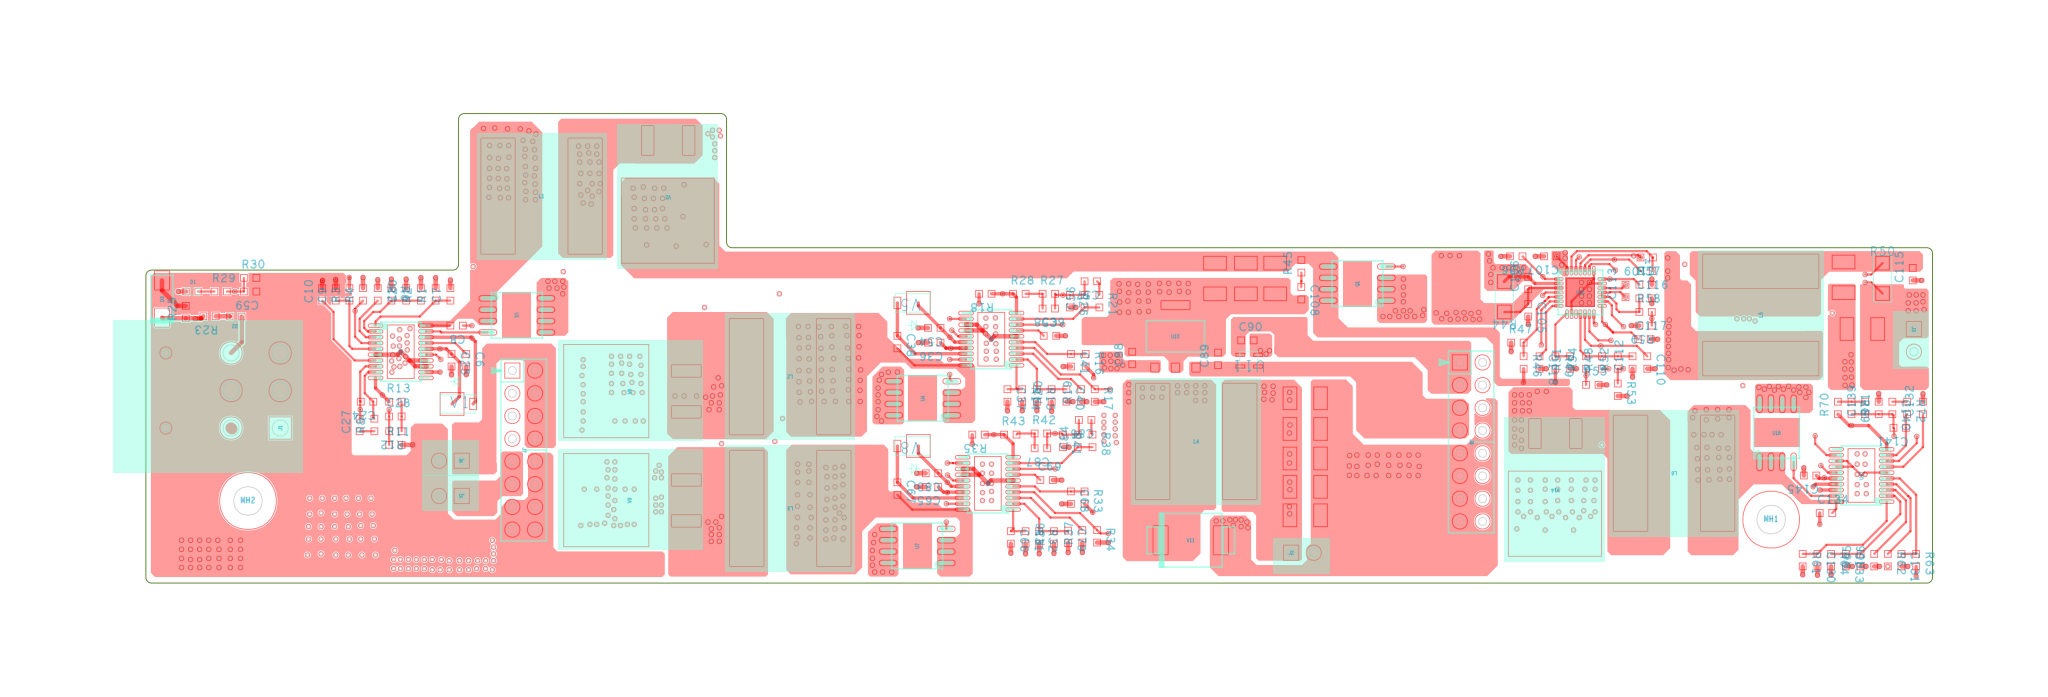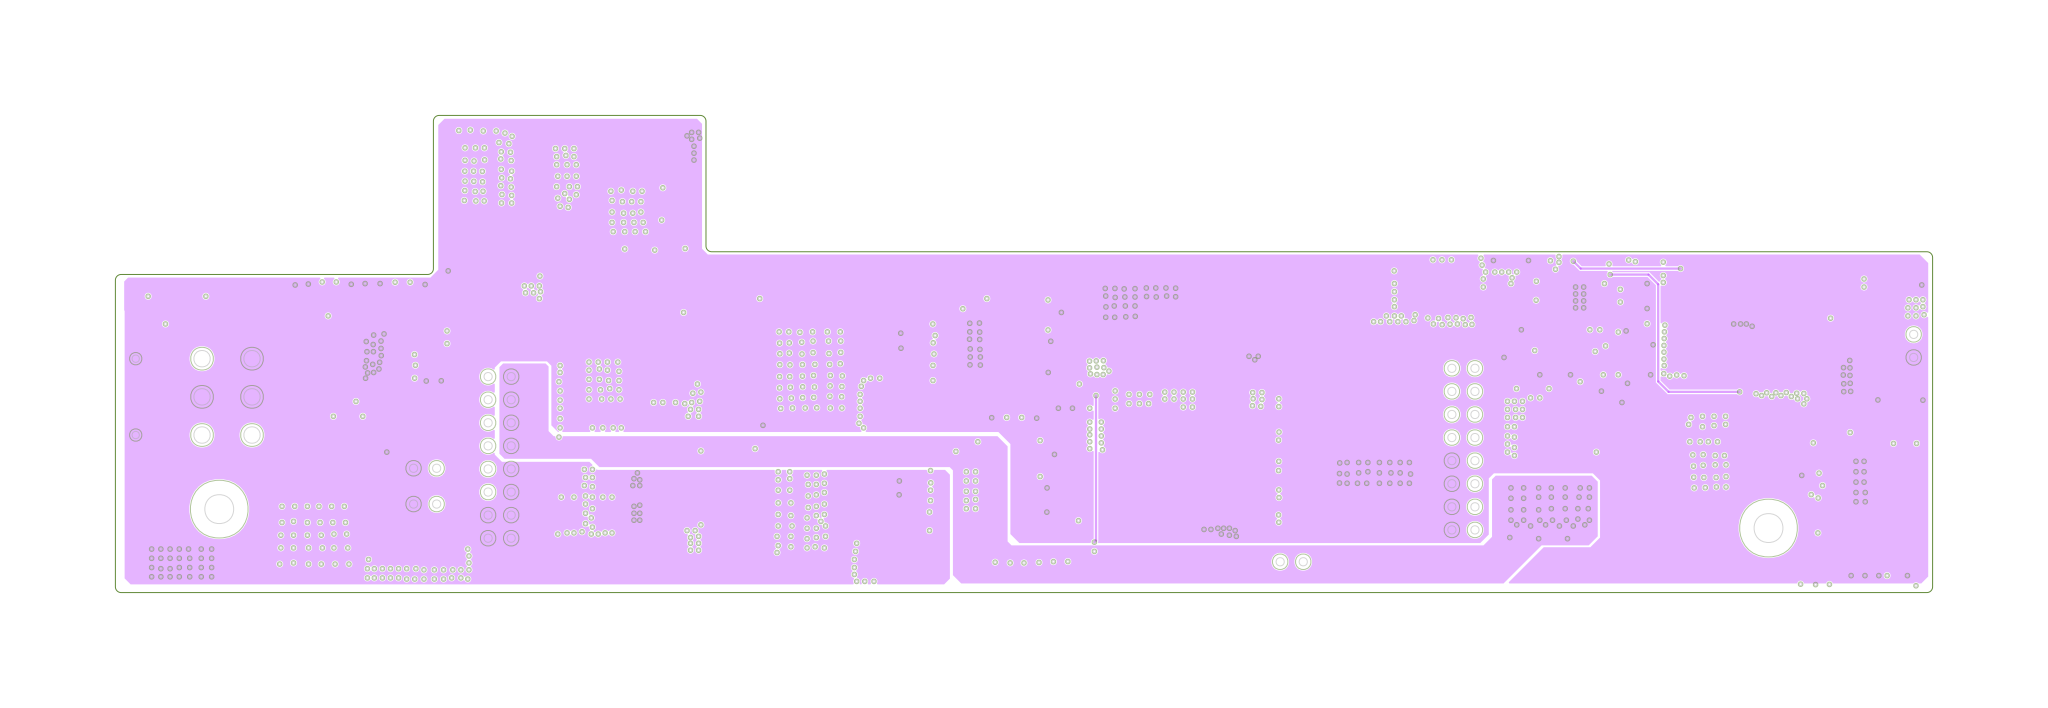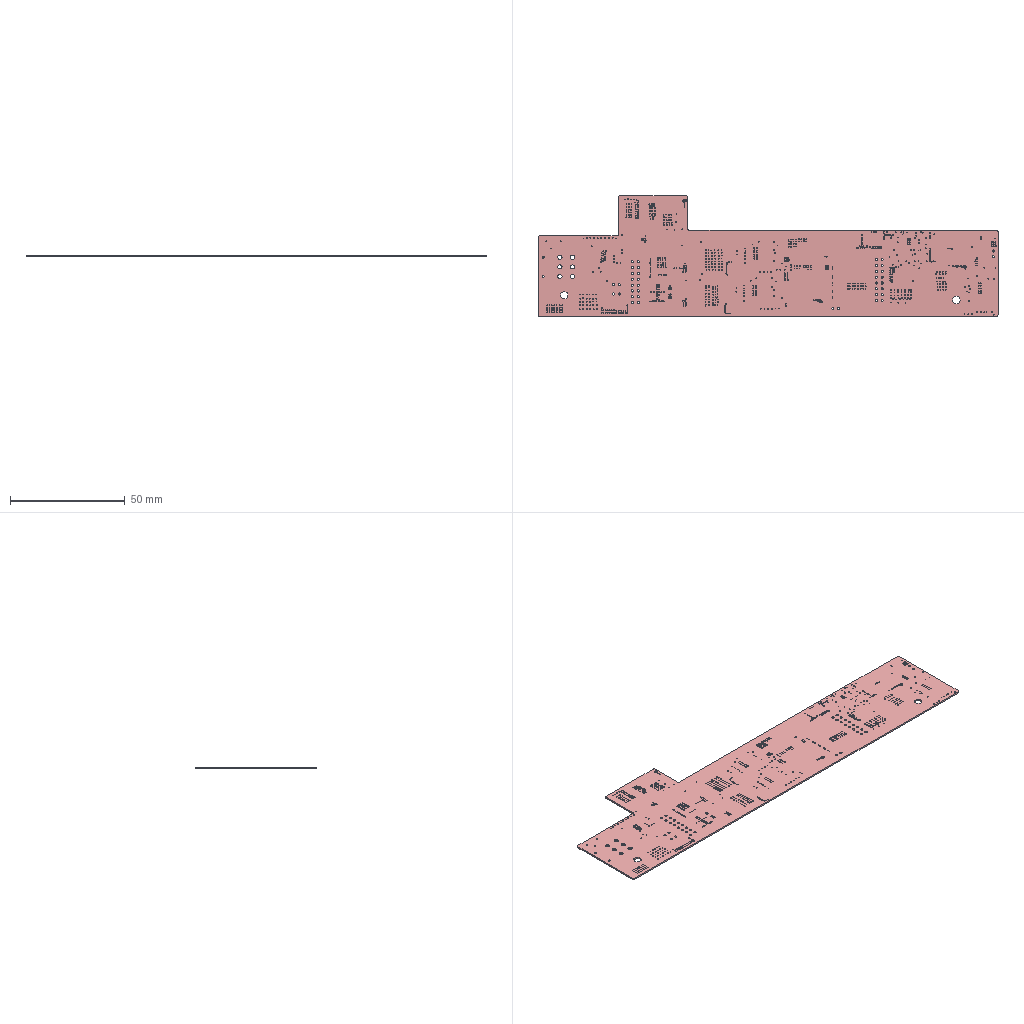Circuit board layout | Cadence Allegro | box 200 x 52.5 x 0.7 mm
Layer stack:
# Cadence Allegro layer stack of  (unit mm; from the constraint file cross-section; dielectric type: 0 not recorded (Allegro does not mark core vs prepreg), 3 surface material)
index,name,kind,layer,copper_thickness_mm,dielectric_type,dielectric_thickness_mm,dielectric_material,dielectric_constant
0,Top Surface,other,,,,,,
1,TOP,copper,TOP,0.0305,,,,
2,Dielectric1,dielectric,,,0,0.2032,FR-4,4.5
3,L2,copper,L2,0.0305,,,,
4,Dielectric2,dielectric,,,0,0.2032,FR-4,4.5
5,L3,copper,L3,0.0305,,,,
6,Dielectric3,dielectric,,,0,0.2032,FR-4,4.5
7,BOTTOM,copper,BOTTOM,0.0305,,,,
8,Bottom Surface,other,,,,,,
# drill layer pairs: low layer,high layer
drill_pair,TOP,BOTTOM
Part placement:
REFDES,COMP_VALUE,SYM_NAME,SYM_X,SYM_Y,SYM_ROTATE,SYM_MIRROR
C1,22uF,C1210,-2818.000,-2737.000,270.000,YES
C6,1uF,C0603,-2585.000,-1952.500,270.000,NO
C7,0.1uF,R0603,-2655.000,-1662.500,90.000,NO
C8,0.1uF,C0603,-2627.500,-1800.000,180.000,NO
C9,330pF,C0603,-3160.000,-1662.500,90.000,NO
C10,0.1uF,C0603,-3220.000,-1662.500,90.000,NO
C11,47uF,C1210,722.000,-1588.000,270.000,NO
C12,47uF,C1210,987.000,-1588.000,270.000,NO
C13,47uF,C1210,-1527.000,-1508.000,90.000,YES
C14,47uF,C1210,858.000,-1588.000,270.000,NO
C15,47uF,C1210,-1561.992,-1041.535,180.000,YES
C16,47uF,C1210,-1561.992,-1179.535,180.000,YES
C17,47uF,C1210,-1561.992,-1317.535,180.000,YES
C18,47uF,C1210,-1797.000,-1508.000,90.000,YES
C19,47uF,C1210,-1662.000,-1508.000,90.000,YES
C20,0.1uF,C0603,-2850.000,-1662.500,90.000,NO
C24,2200pF,C0603,-3022.500,-2135.000,180.000,NO
C25,1uF,C0603,-2650.000,-1952.500,270.000,NO
C26,NO-POP,C0603,-2422.500,-1540.000,0.000,YES
C27,4700pF,C0603,-3055.000,-2237.500,90.000,NO
C28,NO-POP,C0603,-2897.500,-2200.000,0.000,NO
C31,22uF,C1210,-2548.000,-2737.000,270.000,YES
C36,1uF,C0603,-522.500,-1875.000,180.000,NO
C37,0.1uF,R0603,-200.000,-2107.500,270.000,NO
C38,0.1uF,C0603,-685.000,-1872.500,270.000,NO
C39,0.1uF,C0603,-12.500,-1845.000,0.000,NO
C40,0.1uF,R0603,60.000,-2107.500,270.000,NO
C41,330pF,C0603,80.000,-1952.500,270.000,NO
C42,47uF,C1210,-1863.000,-1793.000,270.000,YES
C43,47uF,C1210,-2133.000,-1792.000,270.000,YES
C44,47uF,C1210,-2083.000,-1973.000,0.000,YES
C45,47uF,C1210,-2268.000,-1792.000,270.000,YES
C46,47uF,C1210,-1782.000,-2233.000,90.000,YES
C47,47uF,C1210,-1912.000,-2233.000,90.000,YES
C48,47uF,C1210,-1998.000,-1792.000,270.000,YES
C49,47uF,C1210,-2083.000,-2233.000,0.000,YES
C50,47uF,C1210,-2083.000,-2103.000,0.000,YES
C54,1uF,C0603,-522.500,-1810.000,180.000,NO
C55,0.1uF,C0603,-1177.500,-1700.000,180.000,YES
C56,2200pF,C0603,140.000,-1692.500,90.000,NO
C57,4700pF,C0603,167.500,-1605.000,180.000,NO
C58,0.01uF,C0603,-17.500,-1725.000,180.000,NO
C59,0.1uF,C0603,-3537.500,-1650.000,180.000,NO
C60,22uF,C1210,-2683.000,-2737.000,270.000,YES
C65,1uF,C0603,-532.500,-2510.000,180.000,NO
C66,0.1uF,R0603,-185.000,-2732.500,270.000,NO
C67,0.1uF,C0603,-685.000,-2517.500,270.000,NO
C68,330pF,C0603,80.000,-2557.500,270.000,NO
C69,0.1uF,C0603,-27.500,-2480.000,0.000,NO
C70,47uF,C1210,-1742.000,-2798.000,90.000,YES
C71,47uF,C1210,-1877.000,-2798.000,90.000,YES
C72,47uF,C1210,-2007.000,-2798.000,90.000,YES
C73,47uF,C1210,-2137.000,-2798.000,90.000,YES
C74,47uF,C1210,-2083.000,-2588.000,0.000,YES
C75,47uF,C1210,-1812.000,-2597.000,180.000,YES
C76,47uF,C1210,-1812.000,-2447.000,180.000,YES
C77,47uF,C1210,-1607.000,-2798.000,90.000,YES
C78,47uF,C1210,-2083.000,-2438.000,0.000,YES
C79,0.1uF,R0603,67.500,-2730.000,270.000,NO
C83,1uF,C0603,-532.500,-2450.000,180.000,NO
C84,2200pF,C0603,110.000,-2307.500,90.000,NO
C85,0.1uF,C0603,-1197.500,-2340.000,180.000,YES
C86,4700pF,C0603,142.500,-2215.000,180.000,NO
C87,0.01uF,C0603,-52.500,-2340.000,180.000,NO
C88,0.1uF,C0603,350.000,-1942.500,90.000,NO
C89,0.1uF,C0603,728.000,-1946.500,90.000,NO
C90,0.1uF,C0603,857.500,-1865.000,0.000,NO
C91,47uF/25V,C1210,376.000,-2449.000,90.000,YES
C92,47uF/25V,C1210,239.000,-2448.000,90.000,YES
C93,100uF/10V,C1210,1108.000,-2248.000,0.000,NO
C94,100uF/10V,C1210,1108.000,-2113.000,0.000,NO
C95,100uF/10V,C1210,1108.000,-2628.000,0.000,NO
C96,100uF/10V,C1210,1107.000,-2638.000,180.000,YES
C97,100uF/10V,C1210,1107.000,-2133.000,180.000,YES
C98,100uF/10V,C1210,1107.000,-2383.000,180.000,YES
C99,100uF/10V,C1210,1107.000,-2508.000,180.000,YES
C100,100uF/10V,C1210,1108.000,-2503.000,0.000,NO
C101,100uF/10V,C1210,1108.000,-2378.000,0.000,NO
C102,100uF/10V,C1210,1107.000,-2258.000,180.000,YES
C103,10uF,C1210,3338.000,-1832.000,180.000,YES
C104,10uF,C1210,3338.000,-1962.000,180.000,YES
C105,0.1uF,R0603,2095.000,-1732.500,270.000,NO
C106,0.1uF,R0603,2095.000,-1612.500,90.000,NO
C107,0.1uF,C0603,2192.500,-1495.000,180.000,NO
C108,2.2uF,C0603,1095.000,-1657.500,270.000,NO
C109,0.1uF,C0603,2617.500,-1500.000,180.000,NO
C110,1uF,C0603,2620.000,-1962.500,270.000,NO
C111,10uF,C1210,3492.000,-1583.000,270.000,NO
C112,1uF,C0603,2555.000,-1962.500,90.000,NO
C113,0.1uF,C0603,2524.000,-1647.500,90.000,NO
C114,10uF,C1210,3572.000,-1822.000,180.000,NO
C115,0.1uF,C0603,3790.000,-1573.500,90.000,NO
C116,0.1uF,C0603,2612.500,-1680.000,0.000,NO
C117,100pF,C0603,2607.500,-1860.000,0.000,NO
C118,0.47uF,C0603,2145.000,-1962.500,270.000,NO
C119,47uF,C1210,1611.000,-2626.000,270.000,YES
C120,47uF,C1210,2682.000,-2762.000,90.000,YES
C121,47uF,C1210,1345.000,-2627.000,270.000,YES
C122,47uF,C1210,1478.000,-2626.000,270.000,YES
C123,47uF,C1210,2037.000,-2762.000,90.000,YES
C124,47uF,C1210,2167.000,-2762.000,90.000,YES
C125,47uF,C1210,2297.000,-2762.000,90.000,YES
C126,47uF,C1210,2427.000,-2762.000,90.000,YES
C129,22uF,C1210,3338.000,-2087.000,180.000,YES
C130,0.1uF,R0603,3370.000,-2832.500,270.000,NO
C131,330pF,C0603,3740.000,-2832.500,270.000,NO
C132,0.1uF,C0603,3835.000,-2162.500,90.000,NO
C133,0.1uF,R0603,3495.000,-2832.500,270.000,NO
C134,0.1uF,C0603,3407.500,-2625.000,0.000,NO
C135,0.1uF,C0603,3360.000,-2342.500,90.000,YES
C139,0.01uF,C0603,3580.000,-2162.500,90.000,NO
C140,4700pF,C0603,3700.000,-2162.500,270.000,NO
C141,2200pF,C0603,3732.500,-2250.000,180.000,NO
C142,1uF,C0603,2805.000,-2837.500,90.000,YES
C145,1uF,C0603,3337.500,-2460.000,180.000,NO
C146,47uF,C1210,2557.000,-2762.000,90.000,YES
D1,bat54-02v-gs08,SOD_523,-3793.500,-1650.000,0.000,NO
D2,bat54-02v-gs08,SOD_523,-3600.500,-1760.000,180.000,NO
D3,Zener_ZMM5.1,SOD_123,-3926.000,-1683.110,90.000,NO
D4,bat54-02v-gs08,SOD_523,2616.500,-1560.000,0.000,NO
D5,SMCJ14A-13-F,DO-214AB,-3810.000,-2542.000,90.000,YES
F1,F_6.0A,FUSEFOLDER-OMNI-BLOK,-3182.000,-1987.000,90.000,YES
J1,PoweIn,HDR4MM2_2X3,-3405.000,-2251.000,90.000,NO
J2,+5V,HDR2MM54_1X2,1050.000,-2800.000,0.000,NO
J3,Battery---12V,HDR2MM54_1X2,3795.000,-1815.000,270.000,NO
J5,+5V,HDR2MM54_1X2,-2605.000,-2550.000,180.000,NO
J6,+12V,HDR2MM54_1X2,-2605.000,-2395.000,180.000,NO
J7,HEADER 8X2,HDR2MM54_2X8,-2382.000,-1998.000,270.000,NO
J8,HEADER 8X2,HDR2MM54_2X8,1794.000,-1962.000,270.000,NO
L1,10uH,L-12X12X7,-2253.071,-1230.000,0.000,NO
L2,10uH,L-12X12X7,-1158.071,-2025.000,180.000,NO
L3,10uH,L-12X12X7,-1156.929,-2605.000,180.000,NO
L4,100uH,L-12X14X8,631.929,-2310.000,0.000,NO
L5,10uH,L-12X12X7,3120.000,-1753.071,90.000,NO
L6,10uH,L-12X12X7,2738.071,-2450.000,180.000,NO
MH1,MH_3MM,MHP125-250,3166.000,-2654.000,0.000,NO
MH2,MH_3MM,MHP125-250,-3547.000,-2572.000,0.000,NO
Q1,SI4435BDY,SO_8_PAD,1342.047,-1615.000,90.000,NO
Q2,SI4435BDY,SO_8_PAD,1737.953,-1615.000,270.000,YES
R1,0,R0603,-2720.000,-1662.500,90.000,NO
R2,75K,R0603,-2785.000,-1662.500,90.000,NO
R3,NO-POP,R0603,-3100.000,-1662.500,90.000,NO
R4,1M,R0603,-3040.000,-1662.500,90.000,NO
R6,29.4K,R0603,-2915.000,-1662.500,270.000,NO
R7,16.2K,R0603,-2975.000,-1662.500,270.000,NO
R8,10K,R0603,-2990.000,-2237.500,90.000,NO
R9,0,R0603,-2302.500,-1540.000,0.000,YES
R10,15m_1%_1/2W,R1206,-2361.929,-1615.000,270.000,YES
R11,178,R0603,-2897.500,-2325.000,0.000,NO
R12,2.67K,R0603,-2897.500,-2265.000,180.000,NO
R13,10,R0603,-2897.500,-2135.000,0.000,NO
R14,0,R0603,-135.000,-2107.500,270.000,NO
R15,75K,R0603,-70.000,-2107.500,270.000,NO
R16,NO-POP,R0603,145.000,-1952.500,270.000,NO
R17,1M,R0603,185.000,-2107.500,270.000,NO
R18,NO-POP,R0603,-297.500,-1660.000,180.000,NO
R19,16.2K,R0603,125.000,-2107.500,90.000,NO
R20,29.4K,R0603,-5.000,-2107.500,90.000,NO
R21,10K,R0603,205.000,-1692.500,270.000,NO
R22,0,R0603,-1317.500,-1700.000,180.000,YES
R23,1M 1%,R0603,-3716.500,-1759.000,180.000,NO
R24,15m_1%_1/2W,R1206,-1243.071,-1600.000,90.000,YES
R25,374K 1%,R0603,-3821.000,-1740.500,90.000,NO
R26,309,R0603,75.000,-1692.500,270.000,NO
R27,2.67K,R0603,-17.500,-1660.000,0.000,NO
R28,10,R0603,-147.500,-1660.000,0.000,NO
R29,1M 1%,R0603,-3667.500,-1650.000,0.000,NO
R30,53.6K 1%,R0603,-3537.500,-1590.000,0.000,NO
R31,0,R0603,-120.000,-2732.500,270.000,NO
R32,75K,R0603,-60.000,-2732.500,270.000,NO
R33,NO-POP,R0603,140.000,-2557.500,270.000,NO
R34,1M,R0603,195.000,-2727.500,270.000,NO
R35,NO-POP,R0603,-327.500,-2280.000,180.000,NO
R36,29.4K,R0603,5.000,-2732.500,90.000,NO
R37,16.2K,R0603,130.000,-2727.500,90.000,NO
R38,10K,R0603,175.000,-2307.500,270.000,NO
R39,0,R0603,-1327.500,-2340.000,180.000,YES
R40,15m_1%_1/2W,R1206,-1258.071,-2260.000,90.000,YES
R41,309,R0603,45.000,-2307.500,270.000,NO
R42,2.67K,R0603,-52.500,-2275.000,0.000,NO
R43,10,R0603,-187.500,-2280.000,0.000,NO
R44,10m_1%_1W,R1206,1990.000,-1673.071,180.000,NO
R45,2R,R0603,1095.492,-1539.035,90.000,NO
R46,432K 1%,R0603,2075.000,-1962.500,270.000,NO
R47,66.5K 1%,R0603,2047.500,-1875.000,0.000,NO
R48,10K,R0603,2420.000,-1962.500,90.000,NO
R49,422K 1%,R0603,2215.000,-1962.500,270.000,NO
R50,10m_1%_1W,R1206,3657.000,-1591.929,0.000,NO
R51,71K 1%,R0603,2280.000,-1962.500,90.000,NO
R52,100K,R0603,2490.000,-1962.500,90.000,NO
R53,43K,R0603,2490.000,-2082.500,270.000,NO
R54,100K,R0603,2350.000,-1962.500,90.000,NO
R55,33.6K,R0603,2377.500,-2061.000,0.000,NO
R56,10K,R0603,2042.500,-1495.000,180.000,NO
R57,10K,R0603,2612.500,-1620.000,0.000,NO
R58,1M 1%,R0603,2612.500,-1740.000,0.000,NO
R59,1M 1%,R0603,2612.500,-1800.000,180.000,NO
R60,NO-POP,R0603,2805.000,-2717.500,90.000,YES
R61,0,R0603,3305.000,-2832.500,270.000,NO
R62,1M,R0603,3680.000,-2832.500,270.000,NO
R63,NO-POP,R0603,3805.000,-2832.500,270.000,NO
R64,75K,R0603,3430.000,-2832.500,270.000,NO
R65,29.4K,R0603,3560.000,-2832.500,90.000,NO
R66,16.2K,R0603,3620.000,-2832.500,90.000,NO
R67,15m_1%_1/2W,R1206,3455.000,-2271.929,0.000,YES
R68,0,R0603,3360.000,-2217.500,90.000,YES
R69,2.67K,R0603,3520.000,-2162.500,270.000,NO
R70,10,R0603,3460.000,-2162.500,90.000,NO
R71,309,R0603,3640.000,-2162.500,90.000,NO
R72,10K,R0603,3765.000,-2162.500,270.000,NO
U1,SI7148DP-T1-E3,SO_8_PAD,-2362.047,-1755.000,270.000,NO
U2,LM5118MH/NOPB,TSSOP-20EP,-2873.780,-1915.161,270.000,NO
U3,SI7148DP-T1-E3,SO_8_PAD,-2030.000,-1462.047,0.000,YES
U4,SI7148DP-T1-E3,SO_8_PAD,-572.953,-2120.000,90.000,NO
U5,LM5118MH/NOPB,TSSOP-20EP,-271.220,-1859.839,90.000,NO
U6,SI7148DP-T1-E3,SO_8_PAD,-1610.000,-1912.953,180.000,YES
U7,SI7148DP-T1-E3,SO_8_PAD,-597.953,-2770.000,90.000,NO
U8,LM5118MH/NOPB,TSSOP-20EP,-286.220,-2494.839,90.000,NO
U9,SI7148DP-T1-E3,SO_8_PAD,-1575.000,-2467.953,180.000,YES
U10,UA78M05CDCY,SOT-223,540.551,-1847.402,0.000,NO
U11,XC6215B252NR,SSOT_24,905.000,-1980.000,180.000,NO
U12,LM2576S-5V,TO-263,708.858,-2493.110,180.000,YES
U13,SI4435BDY,SO_8_PAD,3307.047,-1640.000,90.000,YES
U14,SI7148DP-T1-E3,SO_8_PAD,2912.953,-1635.000,270.000,YES
U15,BQ24753ARHDT,QFN28,2325.469,-1654.059,0.000,NO
U16,SI7148DP-T1-E3,SO_8_PAD,2912.047,-1870.000,90.000,YES
U17,LM5118MH/NOPB,TSSOP-20EP,3563.780,-2459.839,90.000,NO
U18,SI7148DP-T1-E3,SO_8_PAD,3190.000,-2272.047,0.000,NO
U19,SI7148DP-T1-E3,SO_8_PAD,2307.047,-2205.000,90.000,YES
V1,MBRM120ET1G,DO_216AA,-2622.500,-2145.000,0.000,NO
V2,MBRD1035CTL,TO-252-2,-1695.157,-1235.394,180.000,NO
V3,MBRD1035CTL,TO-263AB,-2357.362,-1184.606,0.000,YES
V4,MBRD1035CTL,TO-252-2,-3134.843,-2580.394,180.000,YES
V5,MBRM120ET1G,DO_216AA,-617.500,-1700.000,180.000,NO
V6,MBRD1035CTL,TO-252-2,-1865.394,-2089.843,90.000,NO
V7,MBRD1035CTL,TO-263AB,-1094.606,-1977.638,270.000,YES
V8,MBRM120ET1G,DO_216AA,-617.500,-2330.000,180.000,NO
V9,MBRD1035CTL,TO-252-2,-1865.394,-2569.843,90.000,NO
V10,MBRD1035CTL,TO-263AB,-1109.606,-2597.638,270.000,YES
V11,SS34,DO214AB,607.874,-2745.000,0.000,NO
V12,MBRM120ET1G,DO_216AA,3447.500,-2735.000,0.000,YES
V13,MBRD1035CTL,TO-263AB,2929.606,-2312.362,90.000,YES
V14,MBRD1035CTL,TO-252-2,2214.843,-2525.394,180.000,NO
Pad and via stacks:
# Allegro (Cadence) via spans and padstacks; design units: ("mils" 3 1000)
# via spans: padstack,start_layer,end_layer,net_example,count
20RD12,ETCH/TOP,ETCH/BOTTOM,GND,883
# Allegro padstack definitions: name,start_layer,end_layer,drill,plating,holeType,type
25RD,"ETCH/TOP","ETCH/TOP",0.0,"PLATED","none","smd"
84X118REC,"ETCH/TOP","ETCH/TOP",0.0,"PLATED","none","smd"
RX1_15Y3_20R0_10T,"ETCH/TOP","ETCH/TOP",0.0,"PLATED","none","smd"
SR44X40,"ETCH/TOP","ETCH/TOP",0.0,"PLATED","none","smd"
SMD0R74X0R80,"ETCH/TOP","ETCH/TOP",0.0,"PLATED","none","smd"
RX1_45Y1_60R0_10T,"ETCH/TOP","ETCH/TOP",0.0,"PLATED","none","smd"
SR28X30,"ETCH/TOP","ETCH/TOP",0.0,"PLATED","none","smd"
80X128REC,"ETCH/TOP","ETCH/TOP",0.0,"PLATED","none","smd"
59SQ,"ETCH/TOP","ETCH/TOP",0.0,"PLATED","none","smd"
167X150REC,"ETCH/TOP","ETCH/TOP",0.0,"PLATED","none","smd"
RX3_85Y13_00R0_10T,"ETCH/TOP","ETCH/TOP",0.0,"PLATED","none","smd"
115X212REC,"ETCH/TOP","ETCH/TOP",0.0,"PLATED","none","smd"
OX0_61Y2_00T,"ETCH/TOP","ETCH/TOP",0.0,"PLATED","none","smd"
SMDS60,"ETCH/TOP","ETCH/TOP",0.0,"PLATED","none","smd"
SR236X118_NOPASTE,"ETCH/TOP","ETCH/TOP",0.0,"PLATED","none","smd"
OX0_40Y1_65T,"ETCH/TOP","ETCH/TOP",0.0,"PLATED","none","smd"
RX1_20Y2_90R0_10T,"ETCH/TOP","ETCH/TOP",0.0,"PLATED","none","smd"
RX10_95Y12_05R0_10T,"ETCH/TOP","ETCH/TOP",0.0,"PLATED","none","smd"
SR122X122_NOPASTE,"ETCH/TOP","ETCH/TOP",0.0,"PLATED","none","smd"
RX0_30Y0_95R0_10T,"ETCH/TOP","ETCH/TOP",0.0,"PLATED","none","smd"
RX10_51Y7_58R0_10T,"ETCH/TOP","ETCH/TOP",0.0,"PLATED","none","smd"
RX1_40Y3_34R0_10T,"ETCH/TOP","ETCH/TOP",0.0,"PLATED","none","smd"
RX3_25Y1_70R0_10T,"ETCH/TOP","ETCH/TOP",0.0,"PLATED","none","smd"
SR105X100,"ETCH/TOP","ETCH/TOP",0.0,"PLATED","none","smd"
SR30X50,"ETCH/TOP","ETCH/TOP",0.0,"PLATED","none","smd"
RX2_15Y1_70R0_10T,"ETCH/TOP","ETCH/TOP",0.0,"PLATED","none","smd"
RX0_94Y1_01R0_10T,"ETCH/TOP","ETCH/TOP",0.0,"PLATED","none","smd"
RX3_25Y1_01R0_10T,"ETCH/TOP","ETCH/TOP",0.0,"PLATED","none","smd"
SMD_REC_MM35X1,"ETCH/TOP","ETCH/TOP",0.0,"PLATED","none","smd"
PAD2_50D1_80S,"ETCH/TOP","ETCH/BOTTOM",70.87,"PLATED","circle_drill","through"
PAD2_50D1_80,"ETCH/TOP","ETCH/BOTTOM",70.87,"PLATED","circle_drill","through"
PAD1_35D0_80,"ETCH/TOP","ETCH/BOTTOM",31.5,"PLATED","circle_drill","through"
PAD1_70D0_90S,"ETCH/TOP","ETCH/BOTTOM",35.433,"PLATED","circle_drill","through"
PAD1_70D0_90,"ETCH/TOP","ETCH/BOTTOM",35.433,"PLATED","circle_drill","through"
60RD40,"ETCH/TOP","ETCH/BOTTOM",40.0,"PLATED","circle_drill","through"
PAD1_50D0_90,"ETCH/TOP","ETCH/BOTTOM",35.433,"PLATED","circle_drill","through"
250RD125,"ETCH/TOP","ETCH/BOTTOM",125.0,"PLATED","circle_drill","through"
PAD1_70D1_90S,"ETCH/TOP","ETCH/BOTTOM",74.803,"PLATED","circle_drill","through"
PAD1_70D1_90,"ETCH/TOP","ETCH/BOTTOM",74.803,"PLATED","circle_drill","through"
20RD12,"ETCH/TOP","ETCH/BOTTOM",12.0,"PLATED","circle_drill","through"
30RD15,"ETCH/TOP","ETCH/BOTTOM",15.0,"PLATED","circle_drill","through"
FID,"ETCH/TOP","ETCH/TOP",0.0,"PLATED","none","smd"
60X100,"ETCH/TOP","ETCH/TOP",0.0,"PLATED","none","smd"
SMD0603,"ETCH/TOP","ETCH/TOP",0.0,"PLATED","none","smd"
Design rules, without the lines most boards share, first 14 of 26 lines:
# Cadence Allegro design rules of  (from the Constraint Manager export constraints.dcfx, design unit mil; typed fields in mm)
# columns: name | kind | enabled | priority | scope1 | scope2 | descriptor | typed fields (field=value)
# Allegro precedence (priority 1 wins): 1 Region class-to-class, 2 Region class, 3 Region, 4 class-to-class, 5 DiffPair/Bus/NetGroup override, 6 NetClass, 7 constraint set (CSet) default
# per-layer values are written LAYER=value in the descriptor and LAYER:mm in the typed field; a maximum of 0 means no limit set
# --- net classes (and buses / net groups) ---
# (no net classes defined: every net uses the default constraint sets)
# --- track widths, neck and differential-pair gap (physical constraint sets) ---
DEFAULT | PhysicalCSet | enabled | 7 | Design default | All | Physical Constraint (Min Line Width=10mil) (Max Line Width=0mil) (Min Neck Width=5mil) (Max Neck Length=0mil) (DiffPair Primary Gap=0mil) (DiffPair Neck Gap=0mil) (DiffPair Min Space=0mil) (DiffPair Coupled +Tol=0mil) (DiffPair Coupled -Tol=0mil) (Min BB Via Stagger=5mil) (Max BB Via Stagger=0mil) (T-junctions=ANYWHERE) (Pad-pad direct connect=ALL_ALLOWED) (Allowed vias=20RD12, 30RD15, 60RD40) | min_line_width=0.254 min_neck_width=0.127 min_bvia_stagger=0.127 max_bvia_stagger=0 ts_allowed=ANYWHERE diffp_primary_gap=0 diffp_neck_gap=0 max_line_width=0 maximum_neck_length=0 pad_pad_direct_connect=ALL_ALLOWED allow_on_etch_subclass=TRUE diffp_coupled_plus=0 diffp_coupled_minus=0 diffp_min_space=0 vias=20RD12,30RD15,60RD40
# --- clearances: line / pad / via / shape / hole (spacing constraint sets) ---
DEFAULT | SpacingCSet | enabled | 7 | Design default | All | Clearance Constraint (Line-Line=5mil) (Line-SMD Pad=5mil) (Line-Thru Pin=5mil) (Line-Via=5mil) (Line-Shape=5mil) (SMD Pad-SMD Pad=5mil) (Thru Pin-Thru Pin=5mil) (Thru Pin-SMD Pad=5mil) (SMD Pad-Via=10mil) (Thru Pin-Via=5mil) (Via-Via=10mil) (Shape-SMD Pad=5mil) (Shape-Thru Pin=5mil) (Shape-Via=5mil) (Shape-Shape=5mil) (Hole-Hole=10mil) (Hole-Line=10mil) (Hole-Shape=10mil) (BB Via-BB Via=5mil) (uVia-uVia=5mil) | thrupin_to_thrupin_spacing=0.127 thrupin_to_smdpin_spacing=0.127 thrupin_to_thruvia_spacing=0.127 line_to_thrupin_spacing=0.127 thrupin_to_shape_spacing=0.127 smdpin_to_smdpin_spacing=0.127 smdpin_to_thruvia_spacing=0.254 line_to_smdpin_spacing=0.127 shape_to_smdpin_spacing=0.127 thruvia_to_thruvia_spacing=0.254 line_to_thruvia_spacing=0.127 shape_to_thruvia_spacing=0.127 line_to_line_spacing=0.127 line_to_shape_spacing=0.127 shape_to_shape_spacing=0.127 bbv_to_bbv_spacing=0.127 bbv_to_thrupin_spacing=0.127 bbv_to_smdpin_spacing=0.254 bbv_to_thruvia_spacing=0.254 bbv_to_line_spacing=0.254 bbv_to_shape_spacing=0.254 bbv_to_testpin_spacing=0.127 bbv_to_testvia_spacing=0.127 testpin_to_testpin_spacing=0.127 testpin_to_thrupin_spacing=0.127 smdpin_to_testpin_spacing=0.254 testpin_to_thruvia_spacing=0.254 testpin_to_testvia_spacing=0.127 line_to_testpin_spacing=0.127 shape_to_testpin_spacing=0.127 testvia_to_testvia_spacing=0.127 testvia_to_thrupin_spacing=0.127 smdpin_to_testvia_spacing=0.127 testvia_to_thruvia_spacing=0.254 line_to_testvia_spacing=0.254 shape_to_testvia_spacing=0.254 bondpad_to_bondpad_spacing=0.127 thrupin_to_bondpad_spacing=0.127 smdpin_to_bondpad_spacing=0.127 bondpad_to_thruvia_spacing=0.254 bondpad_to_line_spacing=0.254 bondpad_to_shape_spacing=0.127 bondpad_to_bbv_spacing=0.127 bondpad_to_testpin_spacing=0.127 bondpad_to_testvia_spacing=0.127 min_bvia_gap=0.127 hole_to_pin_spacing=0.254 hole_to_via_spacing=0.254 hole_to_line_spacing=0.254 hole_to_shape_spacing=0.254 hole_to_hole_spacing=0.254 mvia_to_mvia_spacing=0.127 mvia_to_thrupin_spacing=1.27 mvia_to_smdpin_spacing=0.127 mvia_to_thruvia_spacing=0.254 mvia_to_bbv_spacing=0.127 mvia_to_line_spacing=0.254 mvia_to_shape_spacing=0.254 mvia_to_testpin_spacing=0.127 mvia_to_testvia_spacing=0.127 bondpad_to_mvia_spacing=0.127 bondpad_to_bondpad_diffp_spc=0.127
DEFAULT | SameNetSpacingCSet | enabled | 7 | Design default | All | Same-Net Clearance (Line-Line=5mil) (Line-SMD Pad=5mil) (Line-Thru Pin=5mil) (Line-Via=5mil) (Line-Shape=5mil) (SMD Pad-SMD Pad=5mil) (Thru Pin-Thru Pin=5mil) (Thru Pin-SMD Pad=5mil) (SMD Pad-Via=5mil) (Thru Pin-Via=5mil) (Via-Via=5mil) (Shape-SMD Pad=5mil) (Shape-Thru Pin=5mil) (Shape-Via=5mil) (Shape-Shape=5mil) (Hole-Hole=8mil) (Hole-Line=8mil) (Hole-Shape=8mil) (BB Via-BB Via=5mil) (uVia-uVia=5mil) | sn_thrupin_to_thrupin_spacing=0.127 sn_thrupin_to_smdpin_spacing=0.127 sn_thrupin_to_thruvia_spacing=0.127 sn_line_to_thrupin_spacing=0.127 sn_thrupin_to_shape_spacing=0.127 sn_smdpin_to_smdpin_spacing=0.127 sn_smdpin_to_thruvia_spacing=0.127 sn_line_to_smdpin_spacing=0.127 sn_shape_to_smdpin_spacing=0.127 sn_thruvia_to_thruvia_spacing=0.127 sn_line_to_thruvia_spacing=0.127 sn_shape_to_thruvia_spacing=0.127 sn_line_to_line_spacing=0.127 sn_line_to_shape_spacing=0.127 sn_shape_to_shape_spacing=0.127 sn_bbv_to_bbv_spacing=0.127 sn_bbv_to_thrupin_spacing=0.127 sn_bbv_to_smdpin_spacing=0.127 sn_bbv_to_thruvia_spacing=0.127 sn_bbv_to_line_spacing=0.127 sn_bbv_to_shape_spacing=0.127 sn_bbv_to_testpin_spacing=0.127 sn_bbv_to_testvia_spacing=0.127 sn_testpin_to_testpin_spacing=0.127 sn_testpin_to_thrupin_spacing=0.127 sn_smdpin_to_testpin_spacing=0.127 sn_testpin_to_thruvia_spacing=0.127 sn_testpin_to_testvia_spacing=0.127 sn_line_to_testpin_spacing=0.127 sn_shape_to_testpin_spacing=0.127 sn_testvia_to_testvia_spacing=0.127 sn_testvia_to_thrupin_spacing=0.127 sn_smdpin_to_testvia_spacing=0.127 sn_testvia_to_thruvia_spacing=0.127 sn_line_to_testvia_spacing=0.127 sn_shape_to_testvia_spacing=0.127 sn_bondpad_to_bondpad_spacing=0.127 sn_thrupin_to_bondpad_spacing=0.127 sn_smdpin_to_bondpad_spacing=0.127 sn_bondpad_to_thruvia_spacing=0.127 sn_bondpad_to_line_spacing=0.127 sn_bondpad_to_shape_spacing=0.127 sn_bondpad_to_bbv_spacing=0.127 sn_bondpad_to_testpin_spacing=0.127 sn_bondpad_to_testvia_spacing=0.127 same_net=TRUE sn_hole_to_pin_spacing=0.2032 sn_hole_to_via_spacing=0.2032 sn_hole_to_line_spacing=0.2032 sn_hole_to_shape_spacing=0.2032 sn_hole_to_hole_spacing=0.2032 sn_mvia_to_mvia_spacing=0.127 sn_mvia_to_thrupin_spacing=0.127 sn_mvia_to_smdpin_spacing=0.127 sn_mvia_to_thruvia_spacing=0.127 sn_mvia_to_bbv_spacing=0.127 sn_mvia_to_line_spacing=0.127 sn_mvia_to_shape_spacing=0.127 sn_mvia_to_testpin_spacing=0.127 sn_mvia_to_testvia_spacing=0.127 sn_bondpad_to_mvia_spacing=0.127
# --- differential pairs (1) ---
DIFFPAIR0 | DiffPair | enabled | 5 | N19167246 | N19167201 | Differential Pair (Primary Gap=0mil) (Min Line Width=10mil) (Physical CSet=DEFAULT) | gap=0 width=0.254 electricalcset=CH
# --- vias and drills (via lists of the physical sets; drills from padstacks.csv) ---